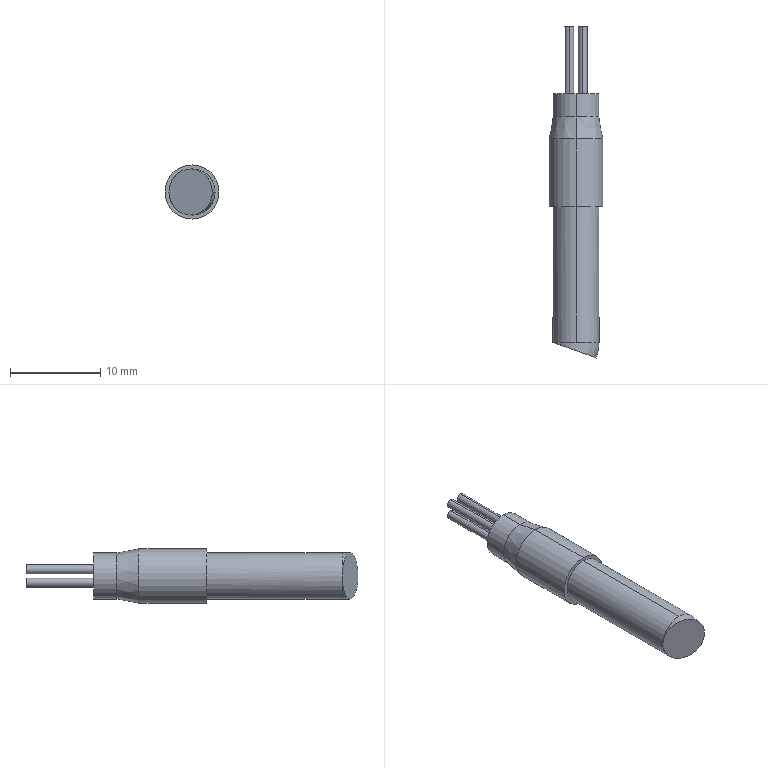Part | SolidWorks | features BaseBody 1 | 1 solid | 25 faces | box 6 x 36.756 x 6 mm | volume 671.876 mm3 | cylinder 14 | plane 7 | spline 2 | cone 2 | commonest cylinder face diameters 1 x8 5.1 x4 6 x2
STEP:
#1=CARTESIAN_POINT('',(2.55,20.,0.));
#2=VERTEX_POINT('',#1);
#3=CARTESIAN_POINT('',(0.,20.,-2.55));
#4=VERTEX_POINT('',#3);
#5=CARTESIAN_POINT('',(0.,20.,0.));
#6=DIRECTION('',(0.,1.,0.));
#7=DIRECTION('',(0.,0.,1.));
#8=AXIS2_PLACEMENT_3D('',#5,#6,#7);
#9=CIRCLE('',#8,2.55);
#10=EDGE_CURVE('',#2,#4,#9,.T.);
#11=ORIENTED_EDGE('',*,*,#10,.T.);
#12=CARTESIAN_POINT('',(0.,35.,-2.55));
#13=VERTEX_POINT('',#12);
#14=CARTESIAN_POINT('',(0.,47.5,-2.55));
#15=DIRECTION('',(0.,1.,0.));
#16=VECTOR('',#15,1000.);
#17=LINE('',#14,#16);
#18=EDGE_CURVE('',#4,#13,#17,.T.);
#19=ORIENTED_EDGE('',*,*,#18,.T.);
#20=CARTESIAN_POINT('',(0.,35.,2.55));
#21=VERTEX_POINT('',#20);
#22=CARTESIAN_POINT('',(0.,35.,0.));
#23=DIRECTION('',(0.,-1.,0.));
#24=DIRECTION('',(0.,0.,1.));
#25=AXIS2_PLACEMENT_3D('',#22,#23,#24);
#26=CIRCLE('',#25,2.55);
#27=EDGE_CURVE('',#13,#21,#26,.T.);
#28=ORIENTED_EDGE('',*,*,#27,.T.);
#29=CARTESIAN_POINT('',(0.,20.,2.55));
#30=VERTEX_POINT('',#29);
#31=CARTESIAN_POINT('',(0.,47.5,2.55));
#32=DIRECTION('',(0.,1.,0.));
#33=VECTOR('',#32,1000.);
#34=LINE('',#31,#33);
#35=EDGE_CURVE('',#30,#21,#34,.T.);
#36=ORIENTED_EDGE('',*,*,#35,.F.);
#37=CARTESIAN_POINT('',(0.,20.,0.));
#38=DIRECTION('',(0.,1.,0.));
#39=DIRECTION('',(0.,0.,1.));
#40=AXIS2_PLACEMENT_3D('',#37,#38,#39);
#41=CIRCLE('',#40,2.55);
#42=EDGE_CURVE('',#30,#2,#41,.T.);
#43=ORIENTED_EDGE('',*,*,#42,.T.);
#44=EDGE_LOOP('',(#11,#19,#28,#36,#43));
#45=FACE_OUTER_BOUND('',#44,.T.);
#46=CARTESIAN_POINT('',(0.,47.5,0.));
#47=DIRECTION('',(0.,1.,0.));
#48=DIRECTION('',(0.,0.,1.));
#49=AXIS2_PLACEMENT_3D('',#46,#47,#48);
#50=CYLINDRICAL_SURFACE('',#49,2.55);
#51=ADVANCED_FACE('',(#45),#50,.T.);
#52=CARTESIAN_POINT('',(2.24,18.244,0.));
#53=VERTEX_POINT('',#52);
#54=CARTESIAN_POINT('',(-2.552,19.988,0.));
#55=VERTEX_POINT('',#54);
#56=CARTESIAN_POINT('',(2.24,18.244,0.));
#57=CARTESIAN_POINT('',(2.24,18.244,-0.1685));
#58=CARTESIAN_POINT('',(2.225,18.249,-0.3342));
#59=CARTESIAN_POINT('',(2.164,18.272,-0.6601));
#60=CARTESIAN_POINT('',(2.118,18.288,-0.822));
#61=CARTESIAN_POINT('',(1.998,18.332,-1.131));
#62=CARTESIAN_POINT('',(1.924,18.359,-1.277));
#63=CARTESIAN_POINT('',(1.75,18.422,-1.555));
#64=CARTESIAN_POINT('',(1.649,18.459,-1.686));
#65=CARTESIAN_POINT('',(1.428,18.54,-1.921));
#66=CARTESIAN_POINT('',(1.307,18.583,-2.027));
#67=CARTESIAN_POINT('',(1.045,18.679,-2.213));
#68=CARTESIAN_POINT('',(0.9055,18.73,-2.292));
#69=CARTESIAN_POINT('',(0.6171,18.835,-2.419));
#70=CARTESIAN_POINT('',(0.4661,18.889,-2.468));
#71=CARTESIAN_POINT('',(0.1567,19.002,-2.534));
#72=CARTESIAN_POINT('',(0.001244,19.059,-2.55));
#73=CARTESIAN_POINT('',(-0.3113,19.172,-2.55));
#74=CARTESIAN_POINT('',(-0.4701,19.23,-2.533));
#75=CARTESIAN_POINT('',(-0.7774,19.342,-2.468));
#76=CARTESIAN_POINT('',(-0.9268,19.396,-2.42));
#77=CARTESIAN_POINT('',(-1.217,19.502,-2.292));
#78=CARTESIAN_POINT('',(-1.357,19.553,-2.213));
#79=CARTESIAN_POINT('',(-1.617,19.648,-2.028));
#80=CARTESIAN_POINT('',(-1.738,19.692,-1.923));
#81=CARTESIAN_POINT('',(-1.962,19.773,-1.685));
#82=CARTESIAN_POINT('',(-2.061,19.809,-1.555));
#83=CARTESIAN_POINT('',(-2.235,19.872,-1.279));
#84=CARTESIAN_POINT('',(-2.31,19.9,-1.13));
#85=CARTESIAN_POINT('',(-2.43,19.944,-0.8212));
#86=CARTESIAN_POINT('',(-2.475,19.96,-0.6622));
#87=CARTESIAN_POINT('',(-2.536,19.982,-0.3354));
#88=CARTESIAN_POINT('',(-2.552,19.988,-0.1664));
#89=CARTESIAN_POINT('',(-2.552,19.988,0.));
#90=B_SPLINE_CURVE_WITH_KNOTS('',3,(#56,#57,#58,#59,#60,#61,#62,#63,#64,#65,#66,#67,#68,#69,#70,#71,#72,#73,#74,#75,#76,#77,#78,#79,#80,#81,#82,#83,#84,#85,#86,#87,#88,#89),.UNSPECIFIED.,.F.,.F.,(4,2,2,2,2,2,2,2,2,2,2,2,2,2,2,2,4),(0.,0.0004983,0.0009966,0.001495,0.001993,0.002491,0.00299,0.003488,0.003986,0.004485,0.004983,0.005481,0.005979,0.006478,0.006976,0.007474,0.007972),.UNSPECIFIED.);
#91=EDGE_CURVE('',#53,#55,#90,.T.);
#92=ORIENTED_EDGE('',*,*,#91,.T.);
#93=CARTESIAN_POINT('',(-2.55,20.,0.));
#94=VERTEX_POINT('',#93);
#95=CARTESIAN_POINT('',(-2.585,20.,0.));
#96=DIRECTION('',(0.,0.,1.));
#97=DIRECTION('',(1.,0.,0.));
#98=AXIS2_PLACEMENT_3D('',#95,#96,#97);
#99=CIRCLE('',#98,0.035);
#100=EDGE_CURVE('',#55,#94,#99,.T.);
#101=ORIENTED_EDGE('',*,*,#100,.T.);
#102=CARTESIAN_POINT('',(0.,20.,0.));
#103=DIRECTION('',(0.,1.,0.));
#104=DIRECTION('',(0.,0.,1.));
#105=AXIS2_PLACEMENT_3D('',#102,#103,#104);
#106=CIRCLE('',#105,2.55);
#107=EDGE_CURVE('',#4,#94,#106,.T.);
#108=ORIENTED_EDGE('',*,*,#107,.F.);
#109=ORIENTED_EDGE('',*,*,#10,.F.);
#110=CARTESIAN_POINT('',(-2.585,20.,0.));
#111=DIRECTION('',(0.,0.,1.));
#112=DIRECTION('',(1.,0.,0.));
#113=AXIS2_PLACEMENT_3D('',#110,#111,#112);
#114=CIRCLE('',#113,5.135);
#115=EDGE_CURVE('',#53,#2,#114,.T.);
#116=ORIENTED_EDGE('',*,*,#115,.F.);
#117=EDGE_LOOP('',(#92,#101,#108,#109,#116));
#118=FACE_OUTER_BOUND('',#117,.T.);
#119=CARTESIAN_POINT('',(2.24,18.244,0.));
#120=CARTESIAN_POINT('',(2.446,18.808,0.));
#121=CARTESIAN_POINT('',(2.55,19.399,0.));
#122=CARTESIAN_POINT('',(2.55,20.,0.));
#123=CARTESIAN_POINT('',(2.24,18.244,-5.1));
#124=CARTESIAN_POINT('',(2.446,18.808,-5.1));
#125=CARTESIAN_POINT('',(2.55,19.399,-5.1));
#126=CARTESIAN_POINT('',(2.55,20.,-5.1));
#127=CARTESIAN_POINT('',(-2.552,19.988,-5.1));
#128=CARTESIAN_POINT('',(-2.551,19.992,-5.1));
#129=CARTESIAN_POINT('',(-2.55,19.996,-5.1));
#130=CARTESIAN_POINT('',(-2.55,20.,-5.1));
#131=CARTESIAN_POINT('',(-2.552,19.988,0.));
#132=CARTESIAN_POINT('',(-2.551,19.992,0.));
#133=CARTESIAN_POINT('',(-2.55,19.996,0.));
#134=CARTESIAN_POINT('',(-2.55,20.,0.));
#135=(BOUNDED_SURFACE()B_SPLINE_SURFACE(3,3,((#119,#120,#121,#122),(#123,#124,#125,#126),(#127,#128,#129,#130),(#131,#132,#133,#134)),.UNSPECIFIED.,.F.,.F.,.F.)B_SPLINE_SURFACE_WITH_KNOTS((4,4),(4,4),(0.,1.),(0.,1.),.UNSPECIFIED.)GEOMETRIC_REPRESENTATION_ITEM()RATIONAL_B_SPLINE_SURFACE(((1.,0.9899,0.9899,1.),(0.3333,0.33,0.33,0.3333),(0.3333,0.33,0.33,0.3333),(1.,0.9899,0.9899,1.)))REPRESENTATION_ITEM('')SURFACE());
#136=ADVANCED_FACE('',(#118),#135,.T.);
#137=CARTESIAN_POINT('',(0.,35.,3.));
#138=VERTEX_POINT('',#137);
#139=CARTESIAN_POINT('',(0.,35.,-3.));
#140=VERTEX_POINT('',#139);
#141=CARTESIAN_POINT('',(0.,35.,0.));
#142=DIRECTION('',(0.,1.,0.));
#143=DIRECTION('',(0.,0.,1.));
#144=AXIS2_PLACEMENT_3D('',#141,#142,#143);
#145=CIRCLE('',#144,3.);
#146=EDGE_CURVE('',#138,#140,#145,.T.);
#147=ORIENTED_EDGE('',*,*,#146,.T.);
#148=CARTESIAN_POINT('',(0.,42.5,-3.));
#149=VERTEX_POINT('',#148);
#150=CARTESIAN_POINT('',(0.,35.,-3.));
#151=DIRECTION('',(0.,1.,0.));
#152=VECTOR('',#151,1000.);
#153=LINE('',#150,#152);
#154=EDGE_CURVE('',#140,#149,#153,.T.);
#155=ORIENTED_EDGE('',*,*,#154,.T.);
#156=CARTESIAN_POINT('',(0.,42.5,3.));
#157=VERTEX_POINT('',#156);
#158=CARTESIAN_POINT('',(0.,42.5,0.));
#159=DIRECTION('',(0.,-1.,0.));
#160=DIRECTION('',(0.,0.,1.));
#161=AXIS2_PLACEMENT_3D('',#158,#159,#160);
#162=CIRCLE('',#161,3.);
#163=EDGE_CURVE('',#149,#157,#162,.T.);
#164=ORIENTED_EDGE('',*,*,#163,.T.);
#165=CARTESIAN_POINT('',(0.,35.,3.));
#166=DIRECTION('',(0.,1.,0.));
#167=VECTOR('',#166,1000.);
#168=LINE('',#165,#167);
#169=EDGE_CURVE('',#138,#157,#168,.T.);
#170=ORIENTED_EDGE('',*,*,#169,.F.);
#171=EDGE_LOOP('',(#147,#155,#164,#170));
#172=FACE_OUTER_BOUND('',#171,.T.);
#173=CARTESIAN_POINT('',(0.,35.,0.));
#174=DIRECTION('',(0.,1.,0.));
#175=DIRECTION('',(0.,0.,1.));
#176=AXIS2_PLACEMENT_3D('',#173,#174,#175);
#177=CYLINDRICAL_SURFACE('',#176,3.);
#178=ADVANCED_FACE('',(#172),#177,.T.);
#179=CARTESIAN_POINT('',(0.,44.926,-2.55));
#180=VERTEX_POINT('',#179);
#181=CARTESIAN_POINT('',(0.,44.926,2.55));
#182=VERTEX_POINT('',#181);
#183=CARTESIAN_POINT('',(0.,44.926,0.));
#184=DIRECTION('',(0.,-1.,0.));
#185=DIRECTION('',(0.,0.,-1.));
#186=AXIS2_PLACEMENT_3D('',#183,#184,#185);
#187=CIRCLE('',#186,2.55);
#188=EDGE_CURVE('',#180,#182,#187,.T.);
#189=ORIENTED_EDGE('',*,*,#188,.T.);
#190=CARTESIAN_POINT('',(0.,42.5,3.));
#191=DIRECTION('',(0.,-0.9832,0.1824));
#192=VECTOR('',#191,1000.);
#193=LINE('',#190,#192);
#194=EDGE_CURVE('',#182,#157,#193,.T.);
#195=ORIENTED_EDGE('',*,*,#194,.T.);
#196=ORIENTED_EDGE('',*,*,#163,.F.);
#197=CARTESIAN_POINT('',(0.,42.5,-3.));
#198=DIRECTION('',(0.,-0.9832,-0.1824));
#199=VECTOR('',#198,1000.);
#200=LINE('',#197,#199);
#201=EDGE_CURVE('',#180,#149,#200,.T.);
#202=ORIENTED_EDGE('',*,*,#201,.F.);
#203=EDGE_LOOP('',(#189,#195,#196,#202));
#204=FACE_OUTER_BOUND('',#203,.T.);
#205=CARTESIAN_POINT('',(0.,42.5,0.));
#206=DIRECTION('',(0.,-1.,0.));
#207=DIRECTION('',(0.,0.,-1.));
#208=AXIS2_PLACEMENT_3D('',#205,#206,#207);
#209=CONICAL_SURFACE('',#208,3.,0.1834);
#210=ADVANCED_FACE('',(#204),#209,.T.);
#211=ORIENTED_EDGE('',*,*,#188,.F.);
#212=CARTESIAN_POINT('',(0.,47.5,-2.55));
#213=VERTEX_POINT('',#212);
#214=CARTESIAN_POINT('',(0.,47.5,-2.55));
#215=DIRECTION('',(0.,1.,0.));
#216=VECTOR('',#215,1000.);
#217=LINE('',#214,#216);
#218=EDGE_CURVE('',#180,#213,#217,.T.);
#219=ORIENTED_EDGE('',*,*,#218,.T.);
#220=CARTESIAN_POINT('',(0.,47.5,2.55));
#221=VERTEX_POINT('',#220);
#222=CARTESIAN_POINT('',(0.,47.5,0.));
#223=DIRECTION('',(0.,-1.,0.));
#224=DIRECTION('',(0.,0.,1.));
#225=AXIS2_PLACEMENT_3D('',#222,#223,#224);
#226=CIRCLE('',#225,2.55);
#227=EDGE_CURVE('',#213,#221,#226,.T.);
#228=ORIENTED_EDGE('',*,*,#227,.T.);
#229=CARTESIAN_POINT('',(0.,47.5,2.55));
#230=DIRECTION('',(0.,1.,0.));
#231=VECTOR('',#230,1000.);
#232=LINE('',#229,#231);
#233=EDGE_CURVE('',#182,#221,#232,.T.);
#234=ORIENTED_EDGE('',*,*,#233,.F.);
#235=EDGE_LOOP('',(#211,#219,#228,#234));
#236=FACE_OUTER_BOUND('',#235,.T.);
#237=CARTESIAN_POINT('',(0.,47.5,0.));
#238=DIRECTION('',(0.,1.,0.));
#239=DIRECTION('',(0.,0.,1.));
#240=AXIS2_PLACEMENT_3D('',#237,#238,#239);
#241=CYLINDRICAL_SURFACE('',#240,2.55);
#242=ADVANCED_FACE('',(#236),#241,.T.);
#243=CARTESIAN_POINT('',(0.75,47.5,-1.25));
#244=VERTEX_POINT('',#243);
#245=CARTESIAN_POINT('',(0.75,47.5,-0.25));
#246=VERTEX_POINT('',#245);
#247=CARTESIAN_POINT('',(0.75,47.5,-0.75));
#248=DIRECTION('',(0.,-1.,0.));
#249=DIRECTION('',(0.,0.,1.));
#250=AXIS2_PLACEMENT_3D('',#247,#248,#249);
#251=CIRCLE('',#250,0.5);
#252=EDGE_CURVE('',#244,#246,#251,.T.);
#253=ORIENTED_EDGE('',*,*,#252,.F.);
#254=CARTESIAN_POINT('',(0.75,55.,-1.25));
#255=VERTEX_POINT('',#254);
#256=CARTESIAN_POINT('',(0.75,55.,-1.25));
#257=DIRECTION('',(0.,1.,0.));
#258=VECTOR('',#257,1000.);
#259=LINE('',#256,#258);
#260=EDGE_CURVE('',#244,#255,#259,.T.);
#261=ORIENTED_EDGE('',*,*,#260,.T.);
#262=CARTESIAN_POINT('',(0.75,55.,-0.25));
#263=VERTEX_POINT('',#262);
#264=CARTESIAN_POINT('',(0.75,55.,-0.75));
#265=DIRECTION('',(0.,-1.,0.));
#266=DIRECTION('',(0.,0.,1.));
#267=AXIS2_PLACEMENT_3D('',#264,#265,#266);
#268=CIRCLE('',#267,0.5);
#269=EDGE_CURVE('',#255,#263,#268,.T.);
#270=ORIENTED_EDGE('',*,*,#269,.T.);
#271=CARTESIAN_POINT('',(0.75,55.,-0.25));
#272=DIRECTION('',(0.,1.,0.));
#273=VECTOR('',#272,1000.);
#274=LINE('',#271,#273);
#275=EDGE_CURVE('',#246,#263,#274,.T.);
#276=ORIENTED_EDGE('',*,*,#275,.F.);
#277=EDGE_LOOP('',(#253,#261,#270,#276));
#278=FACE_OUTER_BOUND('',#277,.T.);
#279=CARTESIAN_POINT('',(0.75,55.,-0.75));
#280=DIRECTION('',(0.,1.,0.));
#281=DIRECTION('',(0.,0.,1.));
#282=AXIS2_PLACEMENT_3D('',#279,#280,#281);
#283=CYLINDRICAL_SURFACE('',#282,0.5);
#284=ADVANCED_FACE('',(#278),#283,.T.);
#285=CARTESIAN_POINT('',(-0.75,47.5,-1.25));
#286=VERTEX_POINT('',#285);
#287=CARTESIAN_POINT('',(-0.75,47.5,-0.25));
#288=VERTEX_POINT('',#287);
#289=CARTESIAN_POINT('',(-0.75,47.5,-0.75));
#290=DIRECTION('',(0.,-1.,0.));
#291=DIRECTION('',(0.,0.,1.));
#292=AXIS2_PLACEMENT_3D('',#289,#290,#291);
#293=CIRCLE('',#292,0.5);
#294=EDGE_CURVE('',#286,#288,#293,.T.);
#295=ORIENTED_EDGE('',*,*,#294,.F.);
#296=CARTESIAN_POINT('',(-0.75,55.,-1.25));
#297=VERTEX_POINT('',#296);
#298=CARTESIAN_POINT('',(-0.75,55.,-1.25));
#299=DIRECTION('',(0.,1.,0.));
#300=VECTOR('',#299,1000.);
#301=LINE('',#298,#300);
#302=EDGE_CURVE('',#286,#297,#301,.T.);
#303=ORIENTED_EDGE('',*,*,#302,.T.);
#304=CARTESIAN_POINT('',(-0.75,55.,-0.25));
#305=VERTEX_POINT('',#304);
#306=CARTESIAN_POINT('',(-0.75,55.,-0.75));
#307=DIRECTION('',(0.,-1.,0.));
#308=DIRECTION('',(0.,0.,1.));
#309=AXIS2_PLACEMENT_3D('',#306,#307,#308);
#310=CIRCLE('',#309,0.5);
#311=EDGE_CURVE('',#297,#305,#310,.T.);
#312=ORIENTED_EDGE('',*,*,#311,.T.);
#313=CARTESIAN_POINT('',(-0.75,55.,-0.25));
#314=DIRECTION('',(0.,1.,0.));
#315=VECTOR('',#314,1000.);
#316=LINE('',#313,#315);
#317=EDGE_CURVE('',#288,#305,#316,.T.);
#318=ORIENTED_EDGE('',*,*,#317,.F.);
#319=EDGE_LOOP('',(#295,#303,#312,#318));
#320=FACE_OUTER_BOUND('',#319,.T.);
#321=CARTESIAN_POINT('',(-0.75,55.,-0.75));
#322=DIRECTION('',(0.,1.,0.));
#323=DIRECTION('',(0.,0.,1.));
#324=AXIS2_PLACEMENT_3D('',#321,#322,#323);
#325=CYLINDRICAL_SURFACE('',#324,0.5);
#326=ADVANCED_FACE('',(#320),#325,.T.);
#327=CARTESIAN_POINT('',(-0.75,47.5,0.25));
#328=VERTEX_POINT('',#327);
#329=CARTESIAN_POINT('',(-0.75,47.5,1.25));
#330=VERTEX_POINT('',#329);
#331=CARTESIAN_POINT('',(-0.75,47.5,0.75));
#332=DIRECTION('',(0.,-1.,0.));
#333=DIRECTION('',(0.,0.,1.));
#334=AXIS2_PLACEMENT_3D('',#331,#332,#333);
#335=CIRCLE('',#334,0.5);
#336=EDGE_CURVE('',#328,#330,#335,.T.);
#337=ORIENTED_EDGE('',*,*,#336,.F.);
#338=CARTESIAN_POINT('',(-0.75,55.,0.25));
#339=VERTEX_POINT('',#338);
#340=CARTESIAN_POINT('',(-0.75,55.,0.25));
#341=DIRECTION('',(0.,1.,0.));
#342=VECTOR('',#341,1000.);
#343=LINE('',#340,#342);
#344=EDGE_CURVE('',#328,#339,#343,.T.);
#345=ORIENTED_EDGE('',*,*,#344,.T.);
#346=CARTESIAN_POINT('',(-0.75,55.,1.25));
#347=VERTEX_POINT('',#346);
#348=CARTESIAN_POINT('',(-0.75,55.,0.75));
#349=DIRECTION('',(0.,-1.,0.));
#350=DIRECTION('',(0.,0.,1.));
#351=AXIS2_PLACEMENT_3D('',#348,#349,#350);
#352=CIRCLE('',#351,0.5);
#353=EDGE_CURVE('',#339,#347,#352,.T.);
#354=ORIENTED_EDGE('',*,*,#353,.T.);
#355=CARTESIAN_POINT('',(-0.75,55.,1.25));
#356=DIRECTION('',(0.,1.,0.));
#357=VECTOR('',#356,1000.);
#358=LINE('',#355,#357);
#359=EDGE_CURVE('',#330,#347,#358,.T.);
#360=ORIENTED_EDGE('',*,*,#359,.F.);
#361=EDGE_LOOP('',(#337,#345,#354,#360));
#362=FACE_OUTER_BOUND('',#361,.T.);
#363=CARTESIAN_POINT('',(-0.75,55.,0.75));
#364=DIRECTION('',(0.,1.,0.));
#365=DIRECTION('',(0.,0.,1.));
#366=AXIS2_PLACEMENT_3D('',#363,#364,#365);
#367=CYLINDRICAL_SURFACE('',#366,0.5);
#368=ADVANCED_FACE('',(#362),#367,.T.);
#369=CARTESIAN_POINT('',(0.75,47.5,0.25));
#370=VERTEX_POINT('',#369);
#371=CARTESIAN_POINT('',(0.75,47.5,1.25));
#372=VERTEX_POINT('',#371);
#373=CARTESIAN_POINT('',(0.75,47.5,0.75));
#374=DIRECTION('',(0.,-1.,0.));
#375=DIRECTION('',(0.,0.,1.));
#376=AXIS2_PLACEMENT_3D('',#373,#374,#375);
#377=CIRCLE('',#376,0.5);
#378=EDGE_CURVE('',#370,#372,#377,.T.);
#379=ORIENTED_EDGE('',*,*,#378,.F.);
#380=CARTESIAN_POINT('',(0.75,55.,0.25));
#381=VERTEX_POINT('',#380);
#382=CARTESIAN_POINT('',(0.75,55.,0.25));
#383=DIRECTION('',(0.,1.,0.));
#384=VECTOR('',#383,1000.);
#385=LINE('',#382,#384);
#386=EDGE_CURVE('',#370,#381,#385,.T.);
#387=ORIENTED_EDGE('',*,*,#386,.T.);
#388=CARTESIAN_POINT('',(0.75,55.,1.25));
#389=VERTEX_POINT('',#388);
#390=CARTESIAN_POINT('',(0.75,55.,0.75));
#391=DIRECTION('',(0.,-1.,0.));
#392=DIRECTION('',(0.,0.,1.));
#393=AXIS2_PLACEMENT_3D('',#390,#391,#392);
#394=CIRCLE('',#393,0.5);
#395=EDGE_CURVE('',#381,#389,#394,.T.);
#396=ORIENTED_EDGE('',*,*,#395,.T.);
#397=CARTESIAN_POINT('',(0.75,55.,1.25));
#398=DIRECTION('',(0.,1.,0.));
#399=VECTOR('',#398,1000.);
#400=LINE('',#397,#399);
#401=EDGE_CURVE('',#372,#389,#400,.T.);
#402=ORIENTED_EDGE('',*,*,#401,.F.);
#403=EDGE_LOOP('',(#379,#387,#396,#402));
#404=FACE_OUTER_BOUND('',#403,.T.);
#405=CARTESIAN_POINT('',(0.75,55.,0.75));
#406=DIRECTION('',(0.,1.,0.));
#407=DIRECTION('',(0.,0.,1.));
#408=AXIS2_PLACEMENT_3D('',#405,#406,#407);
#409=CYLINDRICAL_SURFACE('',#408,0.5);
#410=ADVANCED_FACE('',(#404),#409,.T.);
#411=ORIENTED_EDGE('',*,*,#18,.F.);
#412=ORIENTED_EDGE('',*,*,#107,.T.);
#413=CARTESIAN_POINT('',(0.,20.,0.));
#414=DIRECTION('',(0.,1.,0.));
#415=DIRECTION('',(0.,0.,1.));
#416=AXIS2_PLACEMENT_3D('',#413,#414,#415);
#417=CIRCLE('',#416,2.55);
#418=EDGE_CURVE('',#94,#30,#417,.T.);
#419=ORIENTED_EDGE('',*,*,#418,.T.);
#420=ORIENTED_EDGE('',*,*,#35,.T.);
#421=CARTESIAN_POINT('',(0.,35.,0.));
#422=DIRECTION('',(0.,-1.,0.));
#423=DIRECTION('',(0.,0.,1.));
#424=AXIS2_PLACEMENT_3D('',#421,#422,#423);
#425=CIRCLE('',#424,2.55);
#426=EDGE_CURVE('',#21,#13,#425,.T.);
#427=ORIENTED_EDGE('',*,*,#426,.T.);
#428=EDGE_LOOP('',(#411,#412,#419,#420,#427));
#429=FACE_OUTER_BOUND('',#428,.T.);
#430=CARTESIAN_POINT('',(0.,47.5,0.));
#431=DIRECTION('',(0.,1.,0.));
#432=DIRECTION('',(0.,0.,1.));
#433=AXIS2_PLACEMENT_3D('',#430,#431,#432);
#434=CYLINDRICAL_SURFACE('',#433,2.55);
#435=ADVANCED_FACE('',(#429),#434,.T.);
#436=ORIENTED_EDGE('',*,*,#146,.F.);
#437=CARTESIAN_POINT('',(0.,35.,0.));
#438=DIRECTION('',(0.,1.,0.));
#439=DIRECTION('',(0.,0.,1.));
#440=AXIS2_PLACEMENT_3D('',#437,#438,#439);
#441=CIRCLE('',#440,3.);
#442=EDGE_CURVE('',#140,#138,#441,.T.);
#443=ORIENTED_EDGE('',*,*,#442,.F.);
#444=EDGE_LOOP('',(#436,#443));
#445=FACE_OUTER_BOUND('',#444,.T.);
#446=ORIENTED_EDGE('',*,*,#426,.F.);
#447=ORIENTED_EDGE('',*,*,#27,.F.);
#448=EDGE_LOOP('',(#446,#447));
#449=FACE_BOUND('',#448,.T.);
#450=CARTESIAN_POINT('',(3.,35.,0.));
#451=DIRECTION('',(0.,1.,0.));
#452=DIRECTION('',(0.,0.,1.));
#453=AXIS2_PLACEMENT_3D('',#450,#451,#452);
#454=PLANE('',#453);
#455=ADVANCED_FACE('',(#445,#449),#454,.F.);
#456=ORIENTED_EDGE('',*,*,#100,.F.);
#457=CARTESIAN_POINT('',(-2.552,19.988,0.));
#458=CARTESIAN_POINT('',(-2.552,19.988,0.1664));
#459=CARTESIAN_POINT('',(-2.537,19.983,0.3318));
#460=CARTESIAN_POINT('',(-2.476,19.96,0.6604));
#461=CARTESIAN_POINT('',(-2.43,19.943,0.8216));
#462=CARTESIAN_POINT('',(-2.251,19.878,1.282));
#463=CARTESIAN_POINT('',(-2.072,19.813,1.567));
#464=CARTESIAN_POINT('',(-1.741,19.693,1.919));
#465=CARTESIAN_POINT('',(-1.618,19.648,2.027));
#466=CARTESIAN_POINT('',(-1.357,19.553,2.213));
#467=CARTESIAN_POINT('',(-1.22,19.503,2.291));
#468=CARTESIAN_POINT('',(-0.9301,19.398,2.419));
#469=CARTESIAN_POINT('',(-0.7777,19.342,2.468));
#470=CARTESIAN_POINT('',(-0.4714,19.231,2.533));
#471=CARTESIAN_POINT('',(-0.3159,19.174,2.55));
#472=CARTESIAN_POINT('',(0.00007293,19.059,2.55));
#473=CARTESIAN_POINT('',(0.1564,19.002,2.534));
#474=CARTESIAN_POINT('',(0.4626,18.891,2.469));
#475=CARTESIAN_POINT('',(0.6145,18.835,2.42));
#476=CARTESIAN_POINT('',(0.9051,18.73,2.293));
#477=CARTESIAN_POINT('',(1.043,18.68,2.214));
#478=CARTESIAN_POINT('',(1.303,18.585,2.03));
#479=CARTESIAN_POINT('',(1.427,18.54,1.922));
#480=CARTESIAN_POINT('',(1.648,18.459,1.687));
#481=CARTESIAN_POINT('',(1.747,18.423,1.559));
#482=CARTESIAN_POINT('',(1.922,18.359,1.28));
#483=CARTESIAN_POINT('',(1.997,18.332,1.132));
#484=CARTESIAN_POINT('',(2.177,18.267,0.6716));
#485=CARTESIAN_POINT('',(2.24,18.244,0.3369));
#486=CARTESIAN_POINT('',(2.24,18.244,0.));
#487=B_SPLINE_CURVE_WITH_KNOTS('',3,(#457,#458,#459,#460,#461,#462,#463,#464,#465,#466,#467,#468,#469,#470,#471,#472,#473,#474,#475,#476,#477,#478,#479,#480,#481,#482,#483,#484,#485,#486),.UNSPECIFIED.,.F.,.F.,(4,2,2,2,2,2,2,2,2,2,2,2,2,2,4),(0.007972,0.008471,0.008969,0.009965,0.01046,0.01096,0.01146,0.01196,0.01246,0.01295,0.01345,0.01395,0.01445,0.01495,0.01594),.UNSPECIFIED.);
#488=EDGE_CURVE('',#55,#53,#487,.T.);
#489=ORIENTED_EDGE('',*,*,#488,.T.);
#490=ORIENTED_EDGE('',*,*,#115,.T.);
#491=ORIENTED_EDGE('',*,*,#42,.F.);
#492=ORIENTED_EDGE('',*,*,#418,.F.);
#493=EDGE_LOOP('',(#456,#489,#490,#491,#492));
#494=FACE_OUTER_BOUND('',#493,.T.);
#495=CARTESIAN_POINT('',(-2.552,19.988,0.));
#496=CARTESIAN_POINT('',(-2.551,19.992,0.));
#497=CARTESIAN_POINT('',(-2.55,19.996,0.));
#498=CARTESIAN_POINT('',(-2.55,20.,0.));
#499=CARTESIAN_POINT('',(-2.552,19.988,5.1));
#500=CARTESIAN_POINT('',(-2.551,19.992,5.1));
#501=CARTESIAN_POINT('',(-2.55,19.996,5.1));
#502=CARTESIAN_POINT('',(-2.55,20.,5.1));
#503=CARTESIAN_POINT('',(2.24,18.244,5.1));
#504=CARTESIAN_POINT('',(2.446,18.808,5.1));
#505=CARTESIAN_POINT('',(2.55,19.399,5.1));
#506=CARTESIAN_POINT('',(2.55,20.,5.1));
#507=CARTESIAN_POINT('',(2.24,18.244,0.));
#508=CARTESIAN_POINT('',(2.446,18.808,0.));
#509=CARTESIAN_POINT('',(2.55,19.399,0.));
#510=CARTESIAN_POINT('',(2.55,20.,0.));
#511=(BOUNDED_SURFACE()B_SPLINE_SURFACE(3,3,((#495,#496,#497,#498),(#499,#500,#501,#502),(#503,#504,#505,#506),(#507,#508,#509,#510)),.UNSPECIFIED.,.F.,.F.,.F.)B_SPLINE_SURFACE_WITH_KNOTS((4,4),(4,4),(0.,1.),(0.,1.),.UNSPECIFIED.)GEOMETRIC_REPRESENTATION_ITEM()RATIONAL_B_SPLINE_SURFACE(((1.,0.9899,0.9899,1.),(0.3333,0.33,0.33,0.3333),(0.3333,0.33,0.33,0.3333),(1.,0.9899,0.9899,1.)))REPRESENTATION_ITEM('')SURFACE());
#512=ADVANCED_FACE('',(#494),#511,.T.);
#513=ORIENTED_EDGE('',*,*,#154,.F.);
#514=ORIENTED_EDGE('',*,*,#442,.T.);
#515=ORIENTED_EDGE('',*,*,#169,.T.);
#516=CARTESIAN_POINT('',(0.,42.5,0.));
#517=DIRECTION('',(0.,-1.,0.));
#518=DIRECTION('',(0.,0.,1.));
#519=AXIS2_PLACEMENT_3D('',#516,#517,#518);
#520=CIRCLE('',#519,3.);
#521=EDGE_CURVE('',#157,#149,#520,.T.);
#522=ORIENTED_EDGE('',*,*,#521,.T.);
#523=EDGE_LOOP('',(#513,#514,#515,#522));
#524=FACE_OUTER_BOUND('',#523,.T.);
#525=CARTESIAN_POINT('',(0.,35.,0.));
#526=DIRECTION('',(0.,1.,0.));
#527=DIRECTION('',(0.,0.,1.));
#528=AXIS2_PLACEMENT_3D('',#525,#526,#527);
#529=CYLINDRICAL_SURFACE('',#528,3.);
#530=ADVANCED_FACE('',(#524),#529,.T.);
#531=ORIENTED_EDGE('',*,*,#91,.F.);
#532=ORIENTED_EDGE('',*,*,#488,.F.);
#533=EDGE_LOOP('',(#531,#532));
#534=FACE_OUTER_BOUND('',#533,.T.);
#535=CARTESIAN_POINT('',(-0.1559,19.116,0.));
#536=DIRECTION('',(0.342,0.9397,0.));
#537=DIRECTION('',(-0.9397,0.342,0.));
#538=AXIS2_PLACEMENT_3D('',#535,#536,#537);
#539=PLANE('',#538);
#540=ADVANCED_FACE('',(#534),#539,.F.);
#541=ORIENTED_EDGE('',*,*,#194,.F.);
#542=CARTESIAN_POINT('',(0.,44.926,0.));
#543=DIRECTION('',(0.,-1.,0.));
#544=DIRECTION('',(0.,0.,-1.));
#545=AXIS2_PLACEMENT_3D('',#542,#543,#544);
#546=CIRCLE('',#545,2.55);
#547=EDGE_CURVE('',#182,#180,#546,.T.);
#548=ORIENTED_EDGE('',*,*,#547,.T.);
#549=ORIENTED_EDGE('',*,*,#201,.T.);
#550=ORIENTED_EDGE('',*,*,#521,.F.);
#551=EDGE_LOOP('',(#541,#548,#549,#550));
#552=FACE_OUTER_BOUND('',#551,.T.);
#553=CARTESIAN_POINT('',(0.,42.5,0.));
#554=DIRECTION('',(0.,-1.,0.));
#555=DIRECTION('',(0.,0.,-1.));
#556=AXIS2_PLACEMENT_3D('',#553,#554,#555);
#557=CONICAL_SURFACE('',#556,3.,0.1834);
#558=ADVANCED_FACE('',(#552),#557,.T.);
#559=ORIENTED_EDGE('',*,*,#218,.F.);
#560=ORIENTED_EDGE('',*,*,#547,.F.);
#561=ORIENTED_EDGE('',*,*,#233,.T.);
#562=CARTESIAN_POINT('',(0.,47.5,0.));
#563=DIRECTION('',(0.,-1.,0.));
#564=DIRECTION('',(0.,0.,1.));
#565=AXIS2_PLACEMENT_3D('',#562,#563,#564);
#566=CIRCLE('',#565,2.55);
#567=EDGE_CURVE('',#221,#213,#566,.T.);
#568=ORIENTED_EDGE('',*,*,#567,.T.);
#569=EDGE_LOOP('',(#559,#560,#561,#568));
#570=FACE_OUTER_BOUND('',#569,.T.);
#571=CARTESIAN_POINT('',(0.,47.5,0.));
#572=DIRECTION('',(0.,1.,0.));
#573=DIRECTION('',(0.,0.,1.));
#574=AXIS2_PLACEMENT_3D('',#571,#572,#573);
#575=CYLINDRICAL_SURFACE('',#574,2.55);
#576=ADVANCED_FACE('',(#570),#575,.T.);
#577=ORIENTED_EDGE('',*,*,#567,.F.);
#578=ORIENTED_EDGE('',*,*,#227,.F.);
#579=EDGE_LOOP('',(#577,#578));
#580=FACE_OUTER_BOUND('',#579,.T.);
#581=CARTESIAN_POINT('',(0.75,47.5,-0.75));
#582=DIRECTION('',(0.,-1.,0.));
#583=DIRECTION('',(0.,0.,1.));
#584=AXIS2_PLACEMENT_3D('',#581,#582,#583);
#585=CIRCLE('',#584,0.5);
#586=EDGE_CURVE('',#246,#244,#585,.T.);
#587=ORIENTED_EDGE('',*,*,#586,.T.);
#588=ORIENTED_EDGE('',*,*,#252,.T.);
#589=EDGE_LOOP('',(#587,#588));
#590=FACE_BOUND('',#589,.T.);
#591=CARTESIAN_POINT('',(-0.75,47.5,-0.75));
#592=DIRECTION('',(0.,-1.,0.));
#593=DIRECTION('',(0.,0.,1.));
#594=AXIS2_PLACEMENT_3D('',#591,#592,#593);
#595=CIRCLE('',#594,0.5);
#596=EDGE_CURVE('',#288,#286,#595,.T.);
#597=ORIENTED_EDGE('',*,*,#596,.T.);
#598=ORIENTED_EDGE('',*,*,#294,.T.);
#599=EDGE_LOOP('',(#597,#598));
#600=FACE_BOUND('',#599,.T.);
#601=CARTESIAN_POINT('',(-0.75,47.5,0.75));
#602=DIRECTION('',(0.,-1.,0.));
#603=DIRECTION('',(0.,0.,1.));
#604=AXIS2_PLACEMENT_3D('',#601,#602,#603);
#605=CIRCLE('',#604,0.5);
#606=EDGE_CURVE('',#330,#328,#605,.T.);
#607=ORIENTED_EDGE('',*,*,#606,.T.);
#608=ORIENTED_EDGE('',*,*,#336,.T.);
#609=EDGE_LOOP('',(#607,#608));
#610=FACE_BOUND('',#609,.T.);
#611=CARTESIAN_POINT('',(0.75,47.5,0.75));
#612=DIRECTION('',(0.,-1.,0.));
#613=DIRECTION('',(0.,0.,1.));
#614=AXIS2_PLACEMENT_3D('',#611,#612,#613);
#615=CIRCLE('',#614,0.5);
#616=EDGE_CURVE('',#372,#370,#615,.T.);
#617=ORIENTED_EDGE('',*,*,#616,.T.);
#618=ORIENTED_EDGE('',*,*,#378,.T.);
#619=EDGE_LOOP('',(#617,#618));
#620=FACE_BOUND('',#619,.T.);
#621=CARTESIAN_POINT('',(0.,47.5,0.));
#622=DIRECTION('',(0.,1.,0.));
#623=DIRECTION('',(0.,0.,1.));
#624=AXIS2_PLACEMENT_3D('',#621,#622,#623);
#625=PLANE('',#624);
#626=ADVANCED_FACE('',(#580,#590,#600,#610,#620),#625,.T.);
#627=ORIENTED_EDGE('',*,*,#260,.F.);
#628=ORIENTED_EDGE('',*,*,#586,.F.);
#629=ORIENTED_EDGE('',*,*,#275,.T.);
#630=CARTESIAN_POINT('',(0.75,55.,-0.75));
#631=DIRECTION('',(0.,-1.,0.));
#632=DIRECTION('',(0.,0.,1.));
#633=AXIS2_PLACEMENT_3D('',#630,#631,#632);
#634=CIRCLE('',#633,0.5);
#635=EDGE_CURVE('',#263,#255,#634,.T.);
#636=ORIENTED_EDGE('',*,*,#635,.T.);
#637=EDGE_LOOP('',(#627,#628,#629,#636));
#638=FACE_OUTER_BOUND('',#637,.T.);
#639=CARTESIAN_POINT('',(0.75,55.,-0.75));
#640=DIRECTION('',(0.,1.,0.));
#641=DIRECTION('',(0.,0.,1.));
#642=AXIS2_PLACEMENT_3D('',#639,#640,#641);
#643=CYLINDRICAL_SURFACE('',#642,0.5);
#644=ADVANCED_FACE('',(#638),#643,.T.);
#645=ORIENTED_EDGE('',*,*,#302,.F.);
#646=ORIENTED_EDGE('',*,*,#596,.F.);
#647=ORIENTED_EDGE('',*,*,#317,.T.);
#648=CARTESIAN_POINT('',(-0.75,55.,-0.75));
#649=DIRECTION('',(0.,-1.,0.));
#650=DIRECTION('',(0.,0.,1.));
#651=AXIS2_PLACEMENT_3D('',#648,#649,#650);
#652=CIRCLE('',#651,0.5);
#653=EDGE_CURVE('',#305,#297,#652,.T.);
#654=ORIENTED_EDGE('',*,*,#653,.T.);
#655=EDGE_LOOP('',(#645,#646,#647,#654));
#656=FACE_OUTER_BOUND('',#655,.T.);
#657=CARTESIAN_POINT('',(-0.75,55.,-0.75));
#658=DIRECTION('',(0.,1.,0.));
#659=DIRECTION('',(0.,0.,1.));
#660=AXIS2_PLACEMENT_3D('',#657,#658,#659);
#661=CYLINDRICAL_SURFACE('',#660,0.5);
#662=ADVANCED_FACE('',(#656),#661,.T.);
#663=ORIENTED_EDGE('',*,*,#344,.F.);
#664=ORIENTED_EDGE('',*,*,#606,.F.);
#665=ORIENTED_EDGE('',*,*,#359,.T.);
#666=CARTESIAN_POINT('',(-0.75,55.,0.75));
#667=DIRECTION('',(0.,-1.,0.));
#668=DIRECTION('',(0.,0.,1.));
#669=AXIS2_PLACEMENT_3D('',#666,#667,#668);
#670=CIRCLE('',#669,0.5);
#671=EDGE_CURVE('',#347,#339,#670,.T.);
#672=ORIENTED_EDGE('',*,*,#671,.T.);
#673=EDGE_LOOP('',(#663,#664,#665,#672));
#674=FACE_OUTER_BOUND('',#673,.T.);
#675=CARTESIAN_POINT('',(-0.75,55.,0.75));
#676=DIRECTION('',(0.,1.,0.));
#677=DIRECTION('',(0.,0.,1.));
#678=AXIS2_PLACEMENT_3D('',#675,#676,#677);
#679=CYLINDRICAL_SURFACE('',#678,0.5);
#680=ADVANCED_FACE('',(#674),#679,.T.);
#681=ORIENTED_EDGE('',*,*,#386,.F.);
#682=ORIENTED_EDGE('',*,*,#616,.F.);
#683=ORIENTED_EDGE('',*,*,#401,.T.);
#684=CARTESIAN_POINT('',(0.75,55.,0.75));
#685=DIRECTION('',(0.,-1.,0.));
#686=DIRECTION('',(0.,0.,1.));
#687=AXIS2_PLACEMENT_3D('',#684,#685,#686);
#688=CIRCLE('',#687,0.5);
#689=EDGE_CURVE('',#389,#381,#688,.T.);
#690=ORIENTED_EDGE('',*,*,#689,.T.);
#691=EDGE_LOOP('',(#681,#682,#683,#690));
#692=FACE_OUTER_BOUND('',#691,.T.);
#693=CARTESIAN_POINT('',(0.75,55.,0.75));
#694=DIRECTION('',(0.,1.,0.));
#695=DIRECTION('',(0.,0.,1.));
#696=AXIS2_PLACEMENT_3D('',#693,#694,#695);
#697=CYLINDRICAL_SURFACE('',#696,0.5);
#698=ADVANCED_FACE('',(#692),#697,.T.);
#699=ORIENTED_EDGE('',*,*,#635,.F.);
#700=ORIENTED_EDGE('',*,*,#269,.F.);
#701=EDGE_LOOP('',(#699,#700));
#702=FACE_OUTER_BOUND('',#701,.T.);
#703=CARTESIAN_POINT('',(0.75,55.,-0.75));
#704=DIRECTION('',(0.,1.,0.));
#705=DIRECTION('',(0.,0.,1.));
#706=AXIS2_PLACEMENT_3D('',#703,#704,#705);
#707=PLANE('',#706);
#708=ADVANCED_FACE('',(#702),#707,.T.);
#709=ORIENTED_EDGE('',*,*,#653,.F.);
#710=ORIENTED_EDGE('',*,*,#311,.F.);
#711=EDGE_LOOP('',(#709,#710));
#712=FACE_OUTER_BOUND('',#711,.T.);
#713=CARTESIAN_POINT('',(-0.75,55.,-0.75));
#714=DIRECTION('',(0.,1.,0.));
#715=DIRECTION('',(0.,0.,1.));
#716=AXIS2_PLACEMENT_3D('',#713,#714,#715);
#717=PLANE('',#716);
#718=ADVANCED_FACE('',(#712),#717,.T.);
#719=ORIENTED_EDGE('',*,*,#671,.F.);
#720=ORIENTED_EDGE('',*,*,#353,.F.);
#721=EDGE_LOOP('',(#719,#720));
#722=FACE_OUTER_BOUND('',#721,.T.);
#723=CARTESIAN_POINT('',(-0.75,55.,0.75));
#724=DIRECTION('',(0.,1.,0.));
#725=DIRECTION('',(0.,0.,1.));
#726=AXIS2_PLACEMENT_3D('',#723,#724,#725);
#727=PLANE('',#726);
#728=ADVANCED_FACE('',(#722),#727,.T.);
#729=ORIENTED_EDGE('',*,*,#689,.F.);
#730=ORIENTED_EDGE('',*,*,#395,.F.);
#731=EDGE_LOOP('',(#729,#730));
#732=FACE_OUTER_BOUND('',#731,.T.);
#733=CARTESIAN_POINT('',(0.75,55.,0.75));
#734=DIRECTION('',(0.,1.,0.));
#735=DIRECTION('',(0.,0.,1.));
#736=AXIS2_PLACEMENT_3D('',#733,#734,#735);
#737=PLANE('',#736);
#738=ADVANCED_FACE('',(#732),#737,.T.);
#739=CLOSED_SHELL('',(#51,#136,#178,#210,#242,#284,#326,#368,#410,#435,#455,#512,#530,#540,#558,#576,#626,#644,#662,#680,#698,#708,#718,#728,#738));
#740=MANIFOLD_SOLID_BREP('',#739);
#741=CARTESIAN_POINT('',(0.,0.,0.));
#742=DIRECTION('',(0.,0.,1.));
#743=DIRECTION('',(1.,0.,0.));
#744=AXIS2_PLACEMENT_3D('',#741,#742,#743);
#745=(LENGTH_UNIT()NAMED_UNIT(*)SI_UNIT(.MILLI.,.METRE.));
#746=UNCERTAINTY_MEASURE_WITH_UNIT(LENGTH_MEASURE(0.00001),#745,'','');
#747=(NAMED_UNIT(*)PLANE_ANGLE_UNIT()SI_UNIT($,.RADIAN.));
#748=(NAMED_UNIT(*)SI_UNIT($,.STERADIAN.)SOLID_ANGLE_UNIT());
#749=(GEOMETRIC_REPRESENTATION_CONTEXT(3)GLOBAL_UNCERTAINTY_ASSIGNED_CONTEXT((#746))GLOBAL_UNIT_ASSIGNED_CONTEXT((#745,#747,#748))REPRESENTATION_CONTEXT('',''));
#750=ADVANCED_BREP_SHAPE_REPRESENTATION('',(#740,#744),#749);